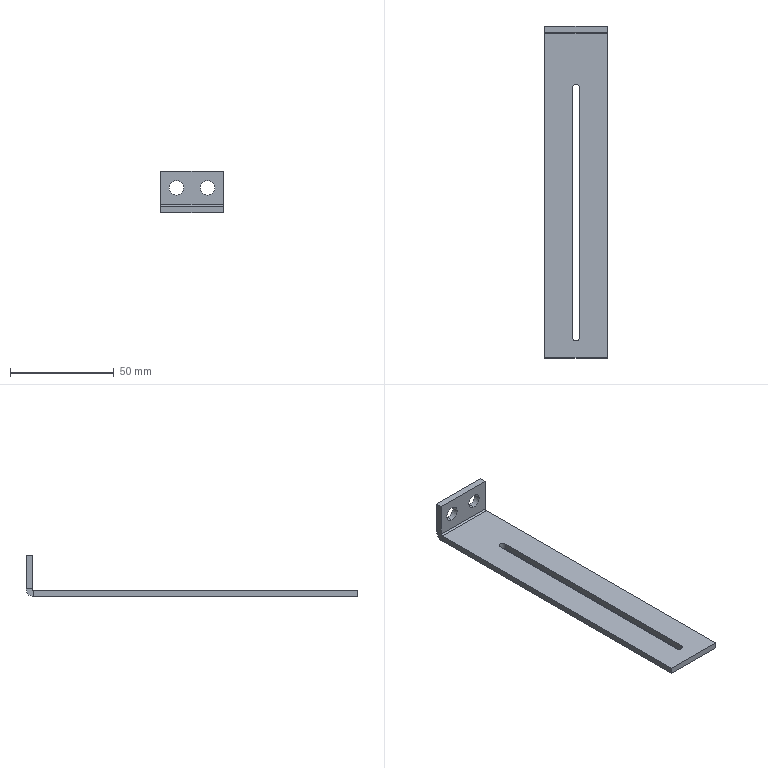Part | STEP file | LM-05-1060A | 1 solid | 22 faces | box 30 x 160 x 20 mm | volume 14324 mm3 | plane 14 | cylinder 8 | commonest cylinder face diameters 7 x4 3.5 x2 1.473 x1 7.473 x1